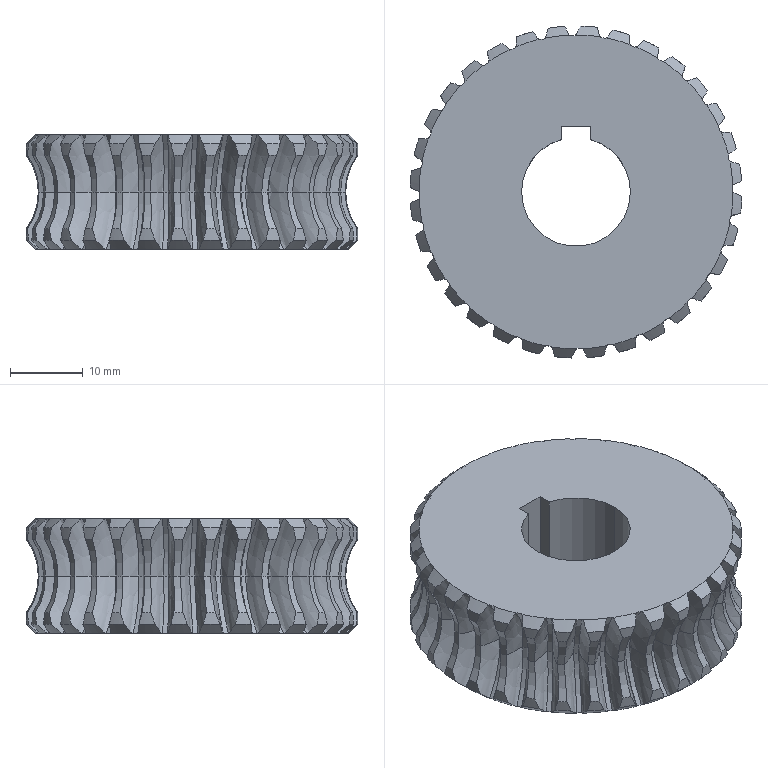Part | SolidWorks | features CirPattern 1, Cut 1, Helix 1, ICE 1, MirrorPattern 1, RefAxis 1, Revolution 1, SweepCut 1 | 1 solid | 394 faces | box 45.721 x 45.721 x 15.75 mm | volume 18731 mm3 | spline 192 | cylinder 67 | cone 66 | torus 64 | plane 5 | commonest cylinder face diameters 45.739 x64 15 x3